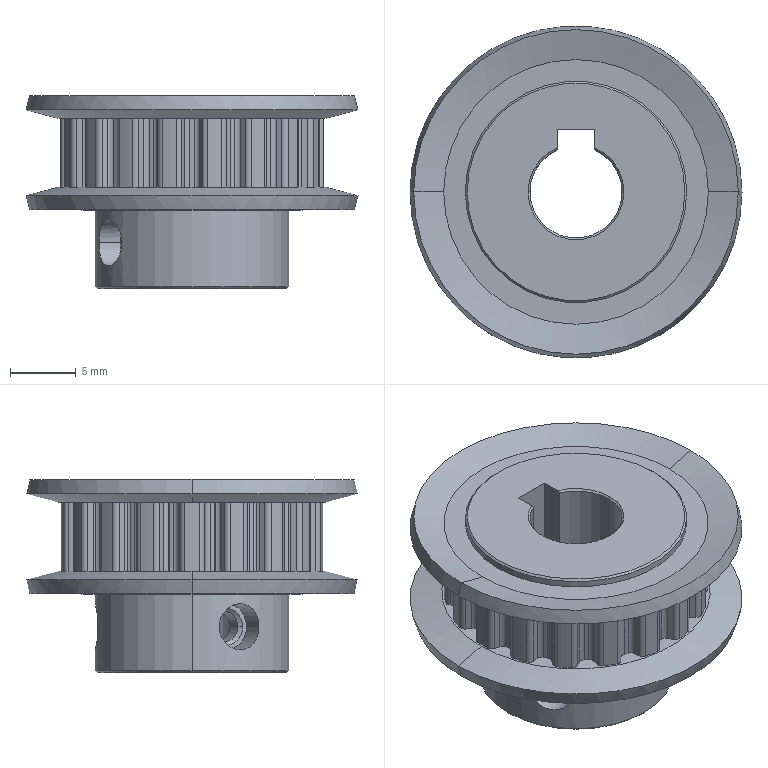Part | SolidWorks | features SplitBody 1 | 1 solid | 217 faces | box 25.2 x 25.2 x 14.7 mm | volume 3255 mm3 | cylinder 141 | plane 48 | cone 28 | commonest cylinder face diameters 0.854 x84 20.02 x19 18.06 x18 2.269 x4 3.5 x4 16.8 x4